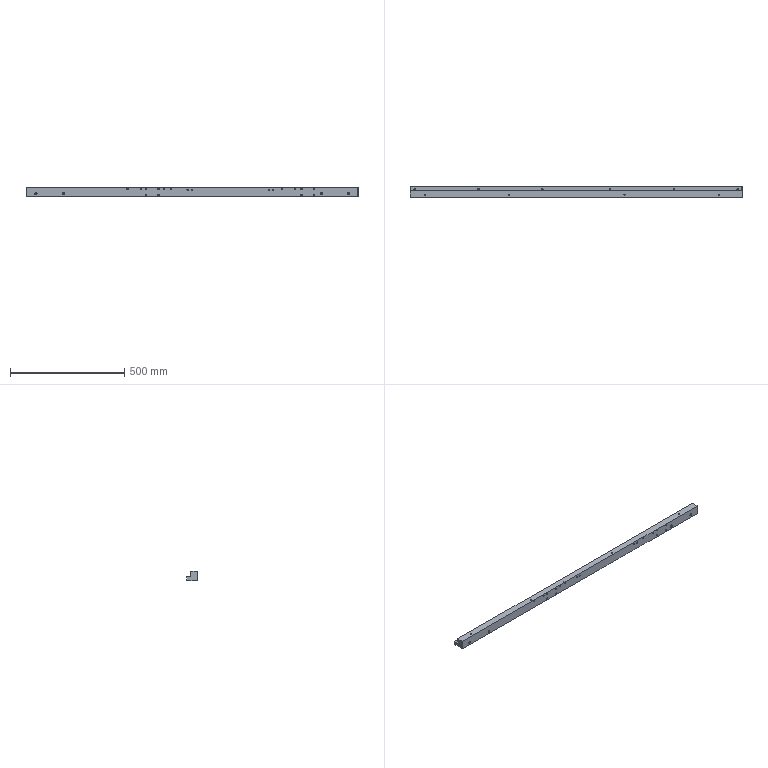Part | STEP file | J013-EBZ05-03-06 | 1 solid | 206 faces | box 1454 x 48 x 40 mm | volume 2137170 mm3 | cylinder 116 | cone 52 | plane 38 | commonest cylinder face diameters 6 x36 5.1 x24 4.2 x20 5 x20 8.6 x8 10 x8